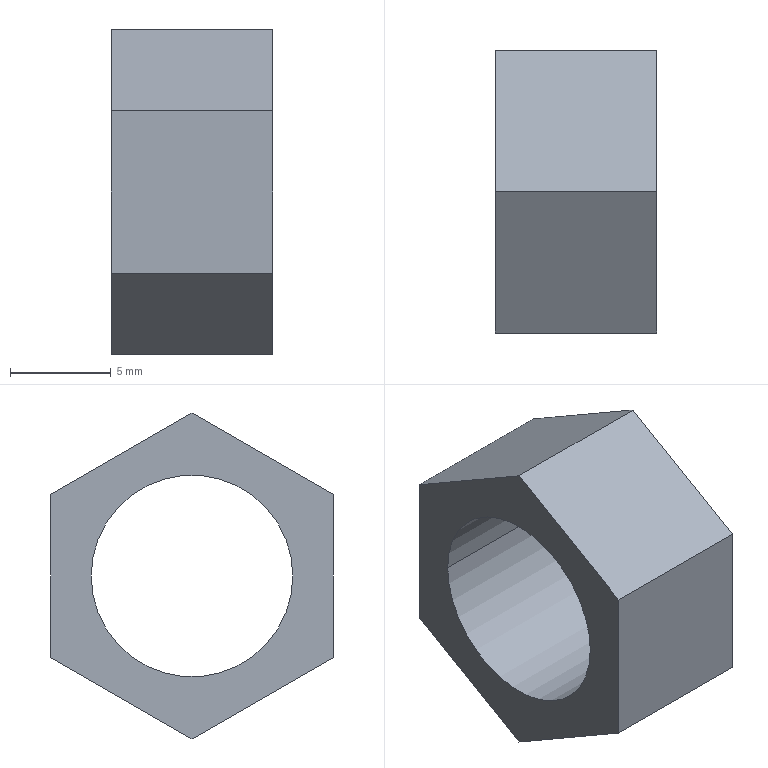Part | NX | features solid 2 | 1 solid | 10 faces | box 8 x 14 x 16.166 mm | volume 729.609 mm3 | plane 8 | cylinder 2 | commonest cylinder face diameters 10 x2
STEP:
#1=CARTESIAN_POINT('',(152.,-64.5,-949.959));
#2=VERTEX_POINT('',#1);
#3=CARTESIAN_POINT('',(152.,-71.5,-945.917));
#4=VERTEX_POINT('',#3);
#5=CARTESIAN_POINT('',(152.,-64.5,-949.959));
#6=DIRECTION('',(0.,-0.866,0.5));
#7=VECTOR('',#6,1000.);
#8=LINE('',#5,#7);
#9=EDGE_CURVE('',#2,#4,#8,.T.);
#10=ORIENTED_EDGE('',*,*,#9,.T.);
#11=CARTESIAN_POINT('',(160.,-71.5,-945.917));
#12=VERTEX_POINT('',#11);
#13=CARTESIAN_POINT('',(160.,-71.5,-945.917));
#14=DIRECTION('',(-1.,0.,0.));
#15=VECTOR('',#14,1000.);
#16=LINE('',#13,#15);
#17=EDGE_CURVE('',#12,#4,#16,.T.);
#18=ORIENTED_EDGE('',*,*,#17,.F.);
#19=CARTESIAN_POINT('',(160.,-64.5,-949.959));
#20=VERTEX_POINT('',#19);
#21=CARTESIAN_POINT('',(160.,-71.5,-945.917));
#22=DIRECTION('',(0.,0.866,-0.5));
#23=VECTOR('',#22,1000.);
#24=LINE('',#21,#23);
#25=EDGE_CURVE('',#12,#20,#24,.T.);
#26=ORIENTED_EDGE('',*,*,#25,.T.);
#27=CARTESIAN_POINT('',(152.,-64.5,-949.959));
#28=DIRECTION('',(1.,0.,0.));
#29=VECTOR('',#28,1000.);
#30=LINE('',#27,#29);
#31=EDGE_CURVE('',#2,#20,#30,.T.);
#32=ORIENTED_EDGE('',*,*,#31,.F.);
#33=EDGE_LOOP('',(#10,#18,#26,#32));
#34=FACE_BOUND('',#33,.T.);
#35=CARTESIAN_POINT('',(152.,-64.5,-949.959));
#36=DIRECTION('',(0.,0.5,0.866));
#37=DIRECTION('',(0.,0.866,-0.5));
#38=AXIS2_PLACEMENT_3D('',#35,#36,#37);
#39=PLANE('',#38);
#40=ADVANCED_FACE('',(#34),#39,.T.);
#41=CARTESIAN_POINT('',(152.,-64.5,-958.041));
#42=VERTEX_POINT('',#41);
#43=CARTESIAN_POINT('',(152.,-64.5,-949.959));
#44=DIRECTION('',(0.,0.,-1.));
#45=VECTOR('',#44,1000.);
#46=LINE('',#43,#45);
#47=EDGE_CURVE('',#2,#42,#46,.T.);
#48=ORIENTED_EDGE('',*,*,#47,.F.);
#49=ORIENTED_EDGE('',*,*,#31,.T.);
#50=CARTESIAN_POINT('',(160.,-64.5,-958.041));
#51=VERTEX_POINT('',#50);
#52=CARTESIAN_POINT('',(160.,-64.5,-949.959));
#53=DIRECTION('',(0.,0.,-1.));
#54=VECTOR('',#53,1000.);
#55=LINE('',#52,#54);
#56=EDGE_CURVE('',#20,#51,#55,.T.);
#57=ORIENTED_EDGE('',*,*,#56,.T.);
#58=CARTESIAN_POINT('',(152.,-64.5,-958.041));
#59=DIRECTION('',(1.,0.,0.));
#60=VECTOR('',#59,1000.);
#61=LINE('',#58,#60);
#62=EDGE_CURVE('',#42,#51,#61,.T.);
#63=ORIENTED_EDGE('',*,*,#62,.F.);
#64=EDGE_LOOP('',(#48,#49,#57,#63));
#65=FACE_BOUND('',#64,.T.);
#66=CARTESIAN_POINT('',(152.,-64.5,-958.041));
#67=DIRECTION('',(0.,1.,0.));
#68=DIRECTION('',(0.,0.,-1.));
#69=AXIS2_PLACEMENT_3D('',#66,#67,#68);
#70=PLANE('',#69);
#71=ADVANCED_FACE('',(#65),#70,.T.);
#72=CARTESIAN_POINT('',(152.,-71.5,-962.083));
#73=VERTEX_POINT('',#72);
#74=CARTESIAN_POINT('',(152.,-71.5,-962.083));
#75=DIRECTION('',(0.,0.866,0.5));
#76=VECTOR('',#75,1000.);
#77=LINE('',#74,#76);
#78=EDGE_CURVE('',#73,#42,#77,.T.);
#79=ORIENTED_EDGE('',*,*,#78,.T.);
#80=ORIENTED_EDGE('',*,*,#62,.T.);
#81=CARTESIAN_POINT('',(160.,-71.5,-962.083));
#82=VERTEX_POINT('',#81);
#83=CARTESIAN_POINT('',(160.,-64.5,-958.041));
#84=DIRECTION('',(0.,-0.866,-0.5));
#85=VECTOR('',#84,1000.);
#86=LINE('',#83,#85);
#87=EDGE_CURVE('',#51,#82,#86,.T.);
#88=ORIENTED_EDGE('',*,*,#87,.T.);
#89=CARTESIAN_POINT('',(152.,-71.5,-962.083));
#90=DIRECTION('',(1.,0.,0.));
#91=VECTOR('',#90,1000.);
#92=LINE('',#89,#91);
#93=EDGE_CURVE('',#73,#82,#92,.T.);
#94=ORIENTED_EDGE('',*,*,#93,.F.);
#95=EDGE_LOOP('',(#79,#80,#88,#94));
#96=FACE_BOUND('',#95,.T.);
#97=CARTESIAN_POINT('',(152.,-71.5,-962.083));
#98=DIRECTION('',(0.,0.5,-0.866));
#99=DIRECTION('',(0.,-0.866,-0.5));
#100=AXIS2_PLACEMENT_3D('',#97,#98,#99);
#101=PLANE('',#100);
#102=ADVANCED_FACE('',(#96),#101,.T.);
#103=CARTESIAN_POINT('',(152.,-78.5,-958.041));
#104=VERTEX_POINT('',#103);
#105=CARTESIAN_POINT('',(152.,-78.5,-958.041));
#106=DIRECTION('',(0.,0.866,-0.5));
#107=VECTOR('',#106,1000.);
#108=LINE('',#105,#107);
#109=EDGE_CURVE('',#104,#73,#108,.T.);
#110=ORIENTED_EDGE('',*,*,#109,.T.);
#111=ORIENTED_EDGE('',*,*,#93,.T.);
#112=CARTESIAN_POINT('',(160.,-78.5,-958.041));
#113=VERTEX_POINT('',#112);
#114=CARTESIAN_POINT('',(160.,-71.5,-962.083));
#115=DIRECTION('',(0.,-0.866,0.5));
#116=VECTOR('',#115,1000.);
#117=LINE('',#114,#116);
#118=EDGE_CURVE('',#82,#113,#117,.T.);
#119=ORIENTED_EDGE('',*,*,#118,.T.);
#120=CARTESIAN_POINT('',(152.,-78.5,-958.041));
#121=DIRECTION('',(1.,0.,0.));
#122=VECTOR('',#121,1000.);
#123=LINE('',#120,#122);
#124=EDGE_CURVE('',#104,#113,#123,.T.);
#125=ORIENTED_EDGE('',*,*,#124,.F.);
#126=EDGE_LOOP('',(#110,#111,#119,#125));
#127=FACE_BOUND('',#126,.T.);
#128=CARTESIAN_POINT('',(152.,-78.5,-958.041));
#129=DIRECTION('',(0.,-0.5,-0.866));
#130=DIRECTION('',(0.,-0.866,0.5));
#131=AXIS2_PLACEMENT_3D('',#128,#129,#130);
#132=PLANE('',#131);
#133=ADVANCED_FACE('',(#127),#132,.T.);
#134=CARTESIAN_POINT('',(152.,-78.5,-949.959));
#135=VERTEX_POINT('',#134);
#136=CARTESIAN_POINT('',(152.,-78.5,-958.041));
#137=DIRECTION('',(0.,0.,1.));
#138=VECTOR('',#137,1000.);
#139=LINE('',#136,#138);
#140=EDGE_CURVE('',#104,#135,#139,.T.);
#141=ORIENTED_EDGE('',*,*,#140,.F.);
#142=ORIENTED_EDGE('',*,*,#124,.T.);
#143=CARTESIAN_POINT('',(160.,-78.5,-949.959));
#144=VERTEX_POINT('',#143);
#145=CARTESIAN_POINT('',(160.,-78.5,-958.041));
#146=DIRECTION('',(0.,0.,1.));
#147=VECTOR('',#146,1000.);
#148=LINE('',#145,#147);
#149=EDGE_CURVE('',#113,#144,#148,.T.);
#150=ORIENTED_EDGE('',*,*,#149,.T.);
#151=CARTESIAN_POINT('',(152.,-78.5,-949.959));
#152=DIRECTION('',(1.,0.,0.));
#153=VECTOR('',#152,1000.);
#154=LINE('',#151,#153);
#155=EDGE_CURVE('',#135,#144,#154,.T.);
#156=ORIENTED_EDGE('',*,*,#155,.F.);
#157=EDGE_LOOP('',(#141,#142,#150,#156));
#158=FACE_BOUND('',#157,.T.);
#159=CARTESIAN_POINT('',(152.,-78.5,-949.959));
#160=DIRECTION('',(0.,-1.,0.));
#161=DIRECTION('',(0.,0.,1.));
#162=AXIS2_PLACEMENT_3D('',#159,#160,#161);
#163=PLANE('',#162);
#164=ADVANCED_FACE('',(#158),#163,.T.);
#165=CARTESIAN_POINT('',(152.,-71.5,-945.917));
#166=DIRECTION('',(0.,-0.866,-0.5));
#167=VECTOR('',#166,1000.);
#168=LINE('',#165,#167);
#169=EDGE_CURVE('',#4,#135,#168,.T.);
#170=ORIENTED_EDGE('',*,*,#169,.T.);
#171=ORIENTED_EDGE('',*,*,#155,.T.);
#172=CARTESIAN_POINT('',(160.,-78.5,-949.959));
#173=DIRECTION('',(0.,0.866,0.5));
#174=VECTOR('',#173,1000.);
#175=LINE('',#172,#174);
#176=EDGE_CURVE('',#144,#12,#175,.T.);
#177=ORIENTED_EDGE('',*,*,#176,.T.);
#178=ORIENTED_EDGE('',*,*,#17,.T.);
#179=EDGE_LOOP('',(#170,#171,#177,#178));
#180=FACE_BOUND('',#179,.T.);
#181=CARTESIAN_POINT('',(152.,-71.5,-945.917));
#182=DIRECTION('',(0.,-0.5,0.866));
#183=DIRECTION('',(0.,0.866,0.5));
#184=AXIS2_PLACEMENT_3D('',#181,#182,#183);
#185=PLANE('',#184);
#186=ADVANCED_FACE('',(#180),#185,.T.);
#187=ORIENTED_EDGE('',*,*,#25,.F.);
#188=ORIENTED_EDGE('',*,*,#176,.F.);
#189=ORIENTED_EDGE('',*,*,#149,.F.);
#190=ORIENTED_EDGE('',*,*,#118,.F.);
#191=ORIENTED_EDGE('',*,*,#87,.F.);
#192=ORIENTED_EDGE('',*,*,#56,.F.);
#193=EDGE_LOOP('',(#187,#188,#189,#190,#191,#192));
#194=FACE_BOUND('',#193,.T.);
#195=CARTESIAN_POINT('',(160.,-76.5,-954.));
#196=VERTEX_POINT('',#195);
#197=CARTESIAN_POINT('',(160.,-66.5,-954.));
#198=VERTEX_POINT('',#197);
#199=CARTESIAN_POINT('',(160.,-71.5,-954.));
#200=DIRECTION('',(1.,0.,0.));
#201=DIRECTION('',(0.,-1.,0.));
#202=AXIS2_PLACEMENT_3D('',#199,#200,#201);
#203=CIRCLE('',#202,5.);
#204=EDGE_CURVE('',#196,#198,#203,.T.);
#205=ORIENTED_EDGE('',*,*,#204,.F.);
#206=CARTESIAN_POINT('',(160.,-71.5,-954.));
#207=DIRECTION('',(1.,0.,0.));
#208=DIRECTION('',(0.,1.,0.));
#209=AXIS2_PLACEMENT_3D('',#206,#207,#208);
#210=CIRCLE('',#209,5.);
#211=EDGE_CURVE('',#198,#196,#210,.T.);
#212=ORIENTED_EDGE('',*,*,#211,.F.);
#213=EDGE_LOOP('',(#205,#212));
#214=FACE_BOUND('',#213,.T.);
#215=CARTESIAN_POINT('',(160.,-71.5,-954.));
#216=DIRECTION('',(1.,0.,0.));
#217=DIRECTION('',(0.,1.,0.));
#218=AXIS2_PLACEMENT_3D('',#215,#216,#217);
#219=PLANE('',#218);
#220=ADVANCED_FACE('',(#194,#214),#219,.T.);
#221=CARTESIAN_POINT('',(152.,-66.5,-954.));
#222=VERTEX_POINT('',#221);
#223=CARTESIAN_POINT('',(160.,-66.5,-954.));
#224=DIRECTION('',(-1.,0.,0.));
#225=VECTOR('',#224,1000.);
#226=LINE('',#223,#225);
#227=EDGE_CURVE('',#222,#198,#226,.F.);
#228=ORIENTED_EDGE('',*,*,#227,.T.);
#229=ORIENTED_EDGE('',*,*,#211,.T.);
#230=CARTESIAN_POINT('',(152.,-76.5,-954.));
#231=VERTEX_POINT('',#230);
#232=CARTESIAN_POINT('',(160.,-76.5,-954.));
#233=DIRECTION('',(-1.,0.,0.));
#234=VECTOR('',#233,1000.);
#235=LINE('',#232,#234);
#236=EDGE_CURVE('',#196,#231,#235,.T.);
#237=ORIENTED_EDGE('',*,*,#236,.T.);
#238=CARTESIAN_POINT('',(152.,-71.5,-954.));
#239=DIRECTION('',(-1.,0.,0.));
#240=DIRECTION('',(0.,-1.,0.));
#241=AXIS2_PLACEMENT_3D('',#238,#239,#240);
#242=CIRCLE('',#241,5.);
#243=EDGE_CURVE('',#231,#222,#242,.T.);
#244=ORIENTED_EDGE('',*,*,#243,.T.);
#245=EDGE_LOOP('',(#228,#229,#237,#244));
#246=FACE_BOUND('',#245,.T.);
#247=CARTESIAN_POINT('',(152.,-71.5,-954.));
#248=DIRECTION('',(1.,0.,0.));
#249=DIRECTION('',(0.,1.,0.));
#250=AXIS2_PLACEMENT_3D('',#247,#248,#249);
#251=CYLINDRICAL_SURFACE('',#250,5.);
#252=ADVANCED_FACE('',(#246),#251,.F.);
#253=ORIENTED_EDGE('',*,*,#109,.F.);
#254=ORIENTED_EDGE('',*,*,#140,.T.);
#255=ORIENTED_EDGE('',*,*,#169,.F.);
#256=ORIENTED_EDGE('',*,*,#9,.F.);
#257=ORIENTED_EDGE('',*,*,#47,.T.);
#258=ORIENTED_EDGE('',*,*,#78,.F.);
#259=EDGE_LOOP('',(#253,#254,#255,#256,#257,#258));
#260=FACE_BOUND('',#259,.T.);
#261=ORIENTED_EDGE('',*,*,#243,.F.);
#262=CARTESIAN_POINT('',(152.,-71.5,-954.));
#263=DIRECTION('',(-1.,0.,0.));
#264=DIRECTION('',(0.,1.,0.));
#265=AXIS2_PLACEMENT_3D('',#262,#263,#264);
#266=CIRCLE('',#265,5.);
#267=EDGE_CURVE('',#222,#231,#266,.T.);
#268=ORIENTED_EDGE('',*,*,#267,.F.);
#269=EDGE_LOOP('',(#261,#268));
#270=FACE_BOUND('',#269,.T.);
#271=CARTESIAN_POINT('',(152.,-71.5,-954.));
#272=DIRECTION('',(1.,0.,0.));
#273=DIRECTION('',(0.,1.,0.));
#274=AXIS2_PLACEMENT_3D('',#271,#272,#273);
#275=PLANE('',#274);
#276=ADVANCED_FACE('',(#260,#270),#275,.F.);
#277=ORIENTED_EDGE('',*,*,#267,.T.);
#278=ORIENTED_EDGE('',*,*,#236,.F.);
#279=ORIENTED_EDGE('',*,*,#204,.T.);
#280=ORIENTED_EDGE('',*,*,#227,.F.);
#281=EDGE_LOOP('',(#277,#278,#279,#280));
#282=FACE_BOUND('',#281,.T.);
#283=CARTESIAN_POINT('',(152.,-71.5,-954.));
#284=DIRECTION('',(1.,0.,0.));
#285=DIRECTION('',(0.,1.,0.));
#286=AXIS2_PLACEMENT_3D('',#283,#284,#285);
#287=CYLINDRICAL_SURFACE('',#286,5.);
#288=ADVANCED_FACE('',(#282),#287,.F.);
#289=CLOSED_SHELL('',(#40,#71,#102,#133,#164,#186,#220,#252,#276,#288));
#290=MANIFOLD_SOLID_BREP('',#289);
#291=(LENGTH_UNIT()NAMED_UNIT(*)SI_UNIT(.MILLI.,.METRE.));
#292=UNCERTAINTY_MEASURE_WITH_UNIT(LENGTH_MEASURE(0.00001),#291,'','');
#293=(NAMED_UNIT(*)PLANE_ANGLE_UNIT()SI_UNIT($,.RADIAN.));
#294=(NAMED_UNIT(*)SI_UNIT($,.STERADIAN.)SOLID_ANGLE_UNIT());
#295=(GEOMETRIC_REPRESENTATION_CONTEXT(3)GLOBAL_UNCERTAINTY_ASSIGNED_CONTEXT((#292))GLOBAL_UNIT_ASSIGNED_CONTEXT((#291,#293,#294))REPRESENTATION_CONTEXT('',''));
#296=ADVANCED_BREP_SHAPE_REPRESENTATION('',(#290),#295);